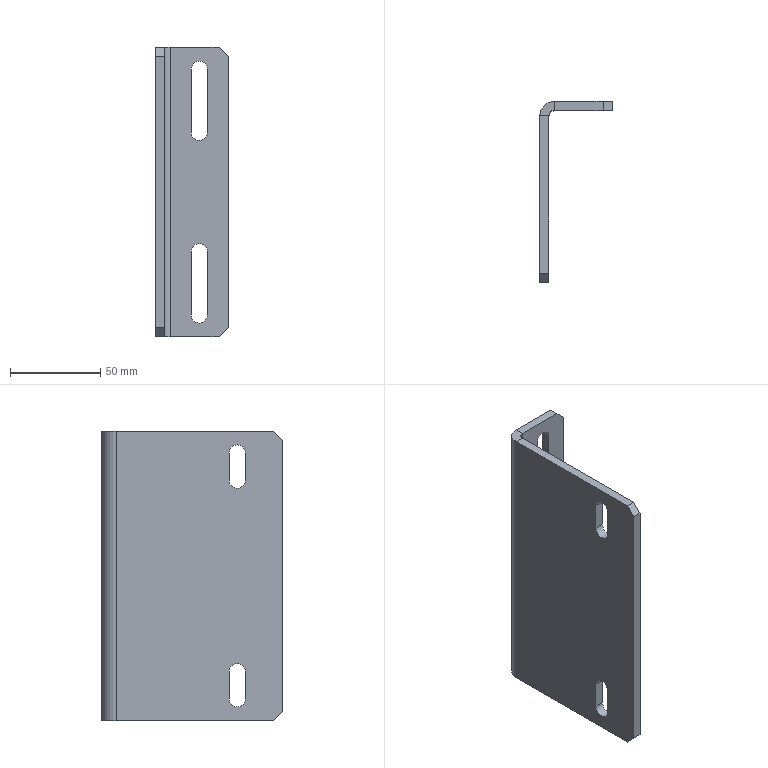Part | SolidWorks | features ICE 2, Chamfer 1, FlatPattern 1, SMBaseFlange 1, SheetMetal 1 | 1 solid | 38 faces | box 40 x 100 x 160 mm | volume 100089 mm3 | plane 24 | cylinder 14 | commonest cylinder face diameters 9 x12 6 x1 16 x1
STEP:
#1=CARTESIAN_POINT('',(28.5,100.,113.));
#2=VERTEX_POINT('',#1);
#3=CARTESIAN_POINT('',(24.,100.,108.5));
#4=VERTEX_POINT('',#3);
#5=CARTESIAN_POINT('',(24.,100.,113.));
#6=DIRECTION('',(0.,1.,0.));
#7=DIRECTION('',(0.,0.,1.));
#8=AXIS2_PLACEMENT_3D('',#5,#6,#7);
#9=CIRCLE('',#8,4.5);
#10=EDGE_CURVE('',#2,#4,#9,.T.);
#11=ORIENTED_EDGE('',*,*,#10,.T.);
#12=CARTESIAN_POINT('',(24.,95.,108.5));
#13=VERTEX_POINT('',#12);
#14=CARTESIAN_POINT('',(24.,105.,108.5));
#15=DIRECTION('',(0.,-1.,0.));
#16=VECTOR('',#15,1000.);
#17=LINE('',#14,#16);
#18=EDGE_CURVE('',#4,#13,#17,.T.);
#19=ORIENTED_EDGE('',*,*,#18,.T.);
#20=CARTESIAN_POINT('',(28.5,95.,113.));
#21=VERTEX_POINT('',#20);
#22=CARTESIAN_POINT('',(24.,95.,113.));
#23=DIRECTION('',(0.,-1.,0.));
#24=DIRECTION('',(0.,0.,1.));
#25=AXIS2_PLACEMENT_3D('',#22,#23,#24);
#26=CIRCLE('',#25,4.5);
#27=EDGE_CURVE('',#13,#21,#26,.T.);
#28=ORIENTED_EDGE('',*,*,#27,.T.);
#29=CARTESIAN_POINT('',(28.5,105.,113.));
#30=DIRECTION('',(0.,-1.,0.));
#31=VECTOR('',#30,1000.);
#32=LINE('',#29,#31);
#33=EDGE_CURVE('',#2,#21,#32,.T.);
#34=ORIENTED_EDGE('',*,*,#33,.F.);
#35=EDGE_LOOP('',(#11,#19,#28,#34));
#36=FACE_OUTER_BOUND('',#35,.T.);
#37=CARTESIAN_POINT('',(24.,105.,113.));
#38=DIRECTION('',(0.,-1.,0.));
#39=DIRECTION('',(0.,0.,-1.));
#40=AXIS2_PLACEMENT_3D('',#37,#38,#39);
#41=CYLINDRICAL_SURFACE('',#40,4.5);
#42=ADVANCED_FACE('',(#36),#41,.F.);
#43=CARTESIAN_POINT('',(28.5,100.,12.));
#44=VERTEX_POINT('',#43);
#45=CARTESIAN_POINT('',(24.,100.,7.5));
#46=VERTEX_POINT('',#45);
#47=CARTESIAN_POINT('',(24.,100.,12.));
#48=DIRECTION('',(0.,1.,0.));
#49=DIRECTION('',(0.,0.,1.));
#50=AXIS2_PLACEMENT_3D('',#47,#48,#49);
#51=CIRCLE('',#50,4.5);
#52=EDGE_CURVE('',#44,#46,#51,.T.);
#53=ORIENTED_EDGE('',*,*,#52,.T.);
#54=CARTESIAN_POINT('',(24.,95.,7.5));
#55=VERTEX_POINT('',#54);
#56=CARTESIAN_POINT('',(24.,105.,7.5));
#57=DIRECTION('',(0.,-1.,0.));
#58=VECTOR('',#57,1000.);
#59=LINE('',#56,#58);
#60=EDGE_CURVE('',#46,#55,#59,.T.);
#61=ORIENTED_EDGE('',*,*,#60,.T.);
#62=CARTESIAN_POINT('',(28.5,95.,12.));
#63=VERTEX_POINT('',#62);
#64=CARTESIAN_POINT('',(24.,95.,12.));
#65=DIRECTION('',(0.,-1.,0.));
#66=DIRECTION('',(0.,0.,-1.));
#67=AXIS2_PLACEMENT_3D('',#64,#65,#66);
#68=CIRCLE('',#67,4.5);
#69=EDGE_CURVE('',#55,#63,#68,.T.);
#70=ORIENTED_EDGE('',*,*,#69,.T.);
#71=CARTESIAN_POINT('',(28.5,105.,12.));
#72=DIRECTION('',(0.,-1.,0.));
#73=VECTOR('',#72,1000.);
#74=LINE('',#71,#73);
#75=EDGE_CURVE('',#44,#63,#74,.T.);
#76=ORIENTED_EDGE('',*,*,#75,.F.);
#77=EDGE_LOOP('',(#53,#61,#70,#76));
#78=FACE_OUTER_BOUND('',#77,.T.);
#79=CARTESIAN_POINT('',(24.,105.,12.));
#80=DIRECTION('',(0.,-1.,0.));
#81=DIRECTION('',(0.,0.,-1.));
#82=AXIS2_PLACEMENT_3D('',#79,#80,#81);
#83=CYLINDRICAL_SURFACE('',#82,4.5);
#84=ADVANCED_FACE('',(#78),#83,.F.);
#85=CARTESIAN_POINT('',(5.,25.,152.5));
#86=VERTEX_POINT('',#85);
#87=CARTESIAN_POINT('',(5.,29.5,148.));
#88=VERTEX_POINT('',#87);
#89=CARTESIAN_POINT('',(5.,25.,148.));
#90=DIRECTION('',(-1.,0.,0.));
#91=DIRECTION('',(0.,0.,1.));
#92=AXIS2_PLACEMENT_3D('',#89,#90,#91);
#93=CIRCLE('',#92,4.5);
#94=EDGE_CURVE('',#86,#88,#93,.T.);
#95=ORIENTED_EDGE('',*,*,#94,.F.);
#96=CARTESIAN_POINT('',(0.,25.,152.5));
#97=VERTEX_POINT('',#96);
#98=CARTESIAN_POINT('',(10.,25.,152.5));
#99=DIRECTION('',(-1.,0.,0.));
#100=VECTOR('',#99,1000.);
#101=LINE('',#98,#100);
#102=EDGE_CURVE('',#86,#97,#101,.T.);
#103=ORIENTED_EDGE('',*,*,#102,.T.);
#104=CARTESIAN_POINT('',(0.,29.5,148.));
#105=VERTEX_POINT('',#104);
#106=CARTESIAN_POINT('',(0.,25.,148.));
#107=DIRECTION('',(-1.,0.,0.));
#108=DIRECTION('',(0.,0.,1.));
#109=AXIS2_PLACEMENT_3D('',#106,#107,#108);
#110=CIRCLE('',#109,4.5);
#111=EDGE_CURVE('',#97,#105,#110,.T.);
#112=ORIENTED_EDGE('',*,*,#111,.T.);
#113=CARTESIAN_POINT('',(10.,29.5,148.));
#114=DIRECTION('',(-1.,0.,0.));
#115=VECTOR('',#114,1000.);
#116=LINE('',#113,#115);
#117=EDGE_CURVE('',#88,#105,#116,.T.);
#118=ORIENTED_EDGE('',*,*,#117,.F.);
#119=EDGE_LOOP('',(#95,#103,#112,#118));
#120=FACE_OUTER_BOUND('',#119,.T.);
#121=CARTESIAN_POINT('',(10.,25.,148.));
#122=DIRECTION('',(-1.,0.,0.));
#123=DIRECTION('',(0.,0.,1.));
#124=AXIS2_PLACEMENT_3D('',#121,#122,#123);
#125=CYLINDRICAL_SURFACE('',#124,4.5);
#126=ADVANCED_FACE('',(#120),#125,.F.);
#127=CARTESIAN_POINT('',(5.,25.,31.5));
#128=VERTEX_POINT('',#127);
#129=CARTESIAN_POINT('',(5.,29.5,27.));
#130=VERTEX_POINT('',#129);
#131=CARTESIAN_POINT('',(5.,25.,27.));
#132=DIRECTION('',(-1.,0.,0.));
#133=DIRECTION('',(0.,0.,1.));
#134=AXIS2_PLACEMENT_3D('',#131,#132,#133);
#135=CIRCLE('',#134,4.5);
#136=EDGE_CURVE('',#128,#130,#135,.T.);
#137=ORIENTED_EDGE('',*,*,#136,.F.);
#138=CARTESIAN_POINT('',(0.,25.,31.5));
#139=VERTEX_POINT('',#138);
#140=CARTESIAN_POINT('',(10.,25.,31.5));
#141=DIRECTION('',(-1.,0.,0.));
#142=VECTOR('',#141,1000.);
#143=LINE('',#140,#142);
#144=EDGE_CURVE('',#128,#139,#143,.T.);
#145=ORIENTED_EDGE('',*,*,#144,.T.);
#146=CARTESIAN_POINT('',(0.,29.5,27.));
#147=VERTEX_POINT('',#146);
#148=CARTESIAN_POINT('',(0.,25.,27.));
#149=DIRECTION('',(-1.,0.,0.));
#150=DIRECTION('',(0.,0.,1.));
#151=AXIS2_PLACEMENT_3D('',#148,#149,#150);
#152=CIRCLE('',#151,4.5);
#153=EDGE_CURVE('',#139,#147,#152,.T.);
#154=ORIENTED_EDGE('',*,*,#153,.T.);
#155=CARTESIAN_POINT('',(10.,29.5,27.));
#156=DIRECTION('',(-1.,0.,0.));
#157=VECTOR('',#156,1000.);
#158=LINE('',#155,#157);
#159=EDGE_CURVE('',#130,#147,#158,.T.);
#160=ORIENTED_EDGE('',*,*,#159,.F.);
#161=EDGE_LOOP('',(#137,#145,#154,#160));
#162=FACE_OUTER_BOUND('',#161,.T.);
#163=CARTESIAN_POINT('',(10.,25.,27.));
#164=DIRECTION('',(-1.,0.,0.));
#165=DIRECTION('',(0.,0.,1.));
#166=AXIS2_PLACEMENT_3D('',#163,#164,#165);
#167=CYLINDRICAL_SURFACE('',#166,4.5);
#168=ADVANCED_FACE('',(#162),#167,.F.);
#169=CARTESIAN_POINT('',(8.,100.,160.));
#170=VERTEX_POINT('',#169);
#171=CARTESIAN_POINT('',(8.,95.,160.));
#172=VERTEX_POINT('',#171);
#173=CARTESIAN_POINT('',(8.,100.,160.));
#174=DIRECTION('',(0.,-1.,0.));
#175=VECTOR('',#174,1000.);
#176=LINE('',#173,#175);
#177=EDGE_CURVE('',#170,#172,#176,.T.);
#178=ORIENTED_EDGE('',*,*,#177,.F.);
#179=CARTESIAN_POINT('',(0.,92.,160.));
#180=VERTEX_POINT('',#179);
#181=CARTESIAN_POINT('',(8.,92.,160.));
#182=DIRECTION('',(0.,0.,-1.));
#183=DIRECTION('',(1.,0.,0.));
#184=AXIS2_PLACEMENT_3D('',#181,#182,#183);
#185=CIRCLE('',#184,8.);
#186=EDGE_CURVE('',#180,#170,#185,.T.);
#187=ORIENTED_EDGE('',*,*,#186,.F.);
#188=CARTESIAN_POINT('',(5.,92.,160.));
#189=VERTEX_POINT('',#188);
#190=CARTESIAN_POINT('',(5.,92.,160.));
#191=DIRECTION('',(-1.,0.,0.));
#192=VECTOR('',#191,1000.);
#193=LINE('',#190,#192);
#194=EDGE_CURVE('',#189,#180,#193,.T.);
#195=ORIENTED_EDGE('',*,*,#194,.F.);
#196=CARTESIAN_POINT('',(8.,92.,160.));
#197=DIRECTION('',(0.,0.,-1.));
#198=DIRECTION('',(1.,0.,0.));
#199=AXIS2_PLACEMENT_3D('',#196,#197,#198);
#200=CIRCLE('',#199,3.);
#201=EDGE_CURVE('',#189,#172,#200,.T.);
#202=ORIENTED_EDGE('',*,*,#201,.T.);
#203=EDGE_LOOP('',(#178,#187,#195,#202));
#204=FACE_OUTER_BOUND('',#203,.T.);
#205=CARTESIAN_POINT('',(8.,100.,160.));
#206=DIRECTION('',(0.,0.,1.));
#207=DIRECTION('',(1.,0.,0.));
#208=AXIS2_PLACEMENT_3D('',#205,#206,#207);
#209=PLANE('',#208);
#210=ADVANCED_FACE('',(#204),#209,.T.);
#211=CARTESIAN_POINT('',(35.,95.,160.));
#212=VERTEX_POINT('',#211);
#213=CARTESIAN_POINT('',(0.,95.,160.));
#214=DIRECTION('',(1.,0.,0.));
#215=VECTOR('',#214,1000.);
#216=LINE('',#213,#215);
#217=EDGE_CURVE('',#172,#212,#216,.T.);
#218=ORIENTED_EDGE('',*,*,#217,.T.);
#219=CARTESIAN_POINT('',(35.,100.,160.));
#220=VERTEX_POINT('',#219);
#221=CARTESIAN_POINT('',(35.,92.,160.));
#222=DIRECTION('',(0.,1.,0.));
#223=VECTOR('',#222,1000.);
#224=LINE('',#221,#223);
#225=EDGE_CURVE('',#212,#220,#224,.T.);
#226=ORIENTED_EDGE('',*,*,#225,.T.);
#227=CARTESIAN_POINT('',(0.,100.,160.));
#228=DIRECTION('',(1.,0.,0.));
#229=VECTOR('',#228,1000.);
#230=LINE('',#227,#229);
#231=EDGE_CURVE('',#170,#220,#230,.T.);
#232=ORIENTED_EDGE('',*,*,#231,.F.);
#233=ORIENTED_EDGE('',*,*,#177,.T.);
#234=EDGE_LOOP('',(#218,#226,#232,#233));
#235=FACE_OUTER_BOUND('',#234,.T.);
#236=CARTESIAN_POINT('',(5.,92.,160.));
#237=DIRECTION('',(0.,0.,1.));
#238=DIRECTION('',(1.,0.,0.));
#239=AXIS2_PLACEMENT_3D('',#236,#237,#238);
#240=PLANE('',#239);
#241=ADVANCED_FACE('',(#235),#240,.T.);
#242=CARTESIAN_POINT('',(0.,92.,0.));
#243=VERTEX_POINT('',#242);
#244=CARTESIAN_POINT('',(5.,92.,0.));
#245=VERTEX_POINT('',#244);
#246=CARTESIAN_POINT('',(0.,92.,0.));
#247=DIRECTION('',(1.,0.,0.));
#248=VECTOR('',#247,1000.);
#249=LINE('',#246,#248);
#250=EDGE_CURVE('',#243,#245,#249,.T.);
#251=ORIENTED_EDGE('',*,*,#250,.F.);
#252=CARTESIAN_POINT('',(8.,100.,0.));
#253=VERTEX_POINT('',#252);
#254=CARTESIAN_POINT('',(8.,92.,0.));
#255=DIRECTION('',(0.,0.,-1.));
#256=DIRECTION('',(1.,0.,0.));
#257=AXIS2_PLACEMENT_3D('',#254,#255,#256);
#258=CIRCLE('',#257,8.);
#259=EDGE_CURVE('',#243,#253,#258,.T.);
#260=ORIENTED_EDGE('',*,*,#259,.T.);
#261=CARTESIAN_POINT('',(8.,95.,0.));
#262=VERTEX_POINT('',#261);
#263=CARTESIAN_POINT('',(8.,95.,0.));
#264=DIRECTION('',(0.,1.,0.));
#265=VECTOR('',#264,1000.);
#266=LINE('',#263,#265);
#267=EDGE_CURVE('',#262,#253,#266,.T.);
#268=ORIENTED_EDGE('',*,*,#267,.F.);
#269=CARTESIAN_POINT('',(8.,92.,0.));
#270=DIRECTION('',(0.,0.,-1.));
#271=DIRECTION('',(1.,0.,0.));
#272=AXIS2_PLACEMENT_3D('',#269,#270,#271);
#273=CIRCLE('',#272,3.);
#274=EDGE_CURVE('',#245,#262,#273,.T.);
#275=ORIENTED_EDGE('',*,*,#274,.F.);
#276=EDGE_LOOP('',(#251,#260,#268,#275));
#277=FACE_OUTER_BOUND('',#276,.T.);
#278=CARTESIAN_POINT('',(0.,92.,0.));
#279=DIRECTION('',(0.,0.,-1.));
#280=DIRECTION('',(-1.,0.,0.));
#281=AXIS2_PLACEMENT_3D('',#278,#279,#280);
#282=PLANE('',#281);
#283=ADVANCED_FACE('',(#277),#282,.T.);
#284=CARTESIAN_POINT('',(5.,5.,0.));
#285=VERTEX_POINT('',#284);
#286=CARTESIAN_POINT('',(5.,0.,0.));
#287=DIRECTION('',(0.,1.,0.));
#288=VECTOR('',#287,1000.);
#289=LINE('',#286,#288);
#290=EDGE_CURVE('',#285,#245,#289,.T.);
#291=ORIENTED_EDGE('',*,*,#290,.F.);
#292=CARTESIAN_POINT('',(0.,5.,0.));
#293=VERTEX_POINT('',#292);
#294=CARTESIAN_POINT('',(8.,5.,0.));
#295=DIRECTION('',(-1.,0.,0.));
#296=VECTOR('',#295,1000.);
#297=LINE('',#294,#296);
#298=EDGE_CURVE('',#285,#293,#297,.T.);
#299=ORIENTED_EDGE('',*,*,#298,.T.);
#300=CARTESIAN_POINT('',(0.,0.,0.));
#301=DIRECTION('',(0.,1.,0.));
#302=VECTOR('',#301,1000.);
#303=LINE('',#300,#302);
#304=EDGE_CURVE('',#293,#243,#303,.T.);
#305=ORIENTED_EDGE('',*,*,#304,.T.);
#306=ORIENTED_EDGE('',*,*,#250,.T.);
#307=EDGE_LOOP('',(#291,#299,#305,#306));
#308=FACE_OUTER_BOUND('',#307,.T.);
#309=CARTESIAN_POINT('',(8.,95.,0.));
#310=DIRECTION('',(0.,0.,-1.));
#311=DIRECTION('',(-1.,0.,0.));
#312=AXIS2_PLACEMENT_3D('',#309,#310,#311);
#313=PLANE('',#312);
#314=ADVANCED_FACE('',(#308),#313,.T.);
#315=CARTESIAN_POINT('',(19.5,95.,148.));
#316=VERTEX_POINT('',#315);
#317=CARTESIAN_POINT('',(19.5,95.,113.));
#318=VERTEX_POINT('',#317);
#319=CARTESIAN_POINT('',(19.5,95.,148.));
#320=DIRECTION('',(0.,0.,-1.));
#321=VECTOR('',#320,1000.);
#322=LINE('',#319,#321);
#323=EDGE_CURVE('',#316,#318,#322,.T.);
#324=ORIENTED_EDGE('',*,*,#323,.F.);
#325=CARTESIAN_POINT('',(28.5,95.,148.));
#326=VERTEX_POINT('',#325);
#327=CARTESIAN_POINT('',(24.,95.,148.));
#328=DIRECTION('',(0.,-1.,0.));
#329=DIRECTION('',(0.,0.,1.));
#330=AXIS2_PLACEMENT_3D('',#327,#328,#329);
#331=CIRCLE('',#330,4.5);
#332=EDGE_CURVE('',#326,#316,#331,.T.);
#333=ORIENTED_EDGE('',*,*,#332,.F.);
#334=CARTESIAN_POINT('',(28.5,95.,148.));
#335=DIRECTION('',(0.,0.,1.));
#336=VECTOR('',#335,1000.);
#337=LINE('',#334,#336);
#338=EDGE_CURVE('',#21,#326,#337,.T.);
#339=ORIENTED_EDGE('',*,*,#338,.F.);
#340=ORIENTED_EDGE('',*,*,#27,.F.);
#341=CARTESIAN_POINT('',(24.,95.,113.));
#342=DIRECTION('',(0.,-1.,0.));
#343=DIRECTION('',(0.,0.,1.));
#344=AXIS2_PLACEMENT_3D('',#341,#342,#343);
#345=CIRCLE('',#344,4.5);
#346=EDGE_CURVE('',#318,#13,#345,.T.);
#347=ORIENTED_EDGE('',*,*,#346,.F.);
#348=EDGE_LOOP('',(#324,#333,#339,#340,#347));
#349=FACE_BOUND('',#348,.T.);
#350=CARTESIAN_POINT('',(28.5,95.,47.));
#351=VERTEX_POINT('',#350);
#352=CARTESIAN_POINT('',(28.5,95.,12.));
#353=DIRECTION('',(0.,0.,1.));
#354=VECTOR('',#353,1000.);
#355=LINE('',#352,#354);
#356=EDGE_CURVE('',#63,#351,#355,.T.);
#357=ORIENTED_EDGE('',*,*,#356,.F.);
#358=ORIENTED_EDGE('',*,*,#69,.F.);
#359=CARTESIAN_POINT('',(19.5,95.,12.));
#360=VERTEX_POINT('',#359);
#361=CARTESIAN_POINT('',(24.,95.,12.));
#362=DIRECTION('',(0.,-1.,0.));
#363=DIRECTION('',(0.,0.,-1.));
#364=AXIS2_PLACEMENT_3D('',#361,#362,#363);
#365=CIRCLE('',#364,4.5);
#366=EDGE_CURVE('',#360,#55,#365,.T.);
#367=ORIENTED_EDGE('',*,*,#366,.F.);
#368=CARTESIAN_POINT('',(19.5,95.,47.));
#369=VERTEX_POINT('',#368);
#370=CARTESIAN_POINT('',(19.5,95.,12.));
#371=DIRECTION('',(0.,0.,-1.));
#372=VECTOR('',#371,1000.);
#373=LINE('',#370,#372);
#374=EDGE_CURVE('',#369,#360,#373,.T.);
#375=ORIENTED_EDGE('',*,*,#374,.F.);
#376=CARTESIAN_POINT('',(24.,95.,47.));
#377=DIRECTION('',(0.,-1.,0.));
#378=DIRECTION('',(0.,0.,-1.));
#379=AXIS2_PLACEMENT_3D('',#376,#377,#378);
#380=CIRCLE('',#379,4.5);
#381=EDGE_CURVE('',#351,#369,#380,.T.);
#382=ORIENTED_EDGE('',*,*,#381,.F.);
#383=EDGE_LOOP('',(#357,#358,#367,#375,#382));
#384=FACE_BOUND('',#383,.T.);
#385=CARTESIAN_POINT('',(35.,95.,0.));
#386=VERTEX_POINT('',#385);
#387=CARTESIAN_POINT('',(0.,95.,0.));
#388=DIRECTION('',(1.,0.,0.));
#389=VECTOR('',#388,1000.);
#390=LINE('',#387,#389);
#391=EDGE_CURVE('',#262,#386,#390,.T.);
#392=ORIENTED_EDGE('',*,*,#391,.T.);
#393=CARTESIAN_POINT('',(40.,95.,5.));
#394=VERTEX_POINT('',#393);
#395=CARTESIAN_POINT('',(35.,95.,0.));
#396=DIRECTION('',(0.7071,0.,0.7071));
#397=VECTOR('',#396,1000.);
#398=LINE('',#395,#397);
#399=EDGE_CURVE('',#386,#394,#398,.T.);
#400=ORIENTED_EDGE('',*,*,#399,.T.);
#401=CARTESIAN_POINT('',(40.,95.,155.));
#402=VERTEX_POINT('',#401);
#403=CARTESIAN_POINT('',(40.,95.,160.));
#404=DIRECTION('',(0.,0.,-1.));
#405=VECTOR('',#404,1000.);
#406=LINE('',#403,#405);
#407=EDGE_CURVE('',#402,#394,#406,.T.);
#408=ORIENTED_EDGE('',*,*,#407,.F.);
#409=CARTESIAN_POINT('',(40.,95.,155.));
#410=DIRECTION('',(-0.7071,0.,0.7071));
#411=VECTOR('',#410,1000.);
#412=LINE('',#409,#411);
#413=EDGE_CURVE('',#402,#212,#412,.T.);
#414=ORIENTED_EDGE('',*,*,#413,.T.);
#415=ORIENTED_EDGE('',*,*,#217,.F.);
#416=CARTESIAN_POINT('',(8.,95.,160.));
#417=DIRECTION('',(0.,0.,-1.));
#418=VECTOR('',#417,1000.);
#419=LINE('',#416,#418);
#420=EDGE_CURVE('',#172,#262,#419,.T.);
#421=ORIENTED_EDGE('',*,*,#420,.T.);
#422=EDGE_LOOP('',(#392,#400,#408,#414,#415,#421));
#423=FACE_OUTER_BOUND('',#422,.T.);
#424=CARTESIAN_POINT('',(0.,95.,160.));
#425=DIRECTION('',(0.,1.,0.));
#426=DIRECTION('',(0.,0.,1.));
#427=AXIS2_PLACEMENT_3D('',#424,#425,#426);
#428=PLANE('',#427);
#429=ADVANCED_FACE('',(#349,#384,#423),#428,.F.);
#430=ORIENTED_EDGE('',*,*,#407,.T.);
#431=CARTESIAN_POINT('',(40.,100.,5.));
#432=VERTEX_POINT('',#431);
#433=CARTESIAN_POINT('',(40.,100.,5.));
#434=DIRECTION('',(0.,1.,0.));
#435=VECTOR('',#434,1000.);
#436=LINE('',#433,#435);
#437=EDGE_CURVE('',#394,#432,#436,.T.);
#438=ORIENTED_EDGE('',*,*,#437,.T.);
#439=CARTESIAN_POINT('',(40.,100.,155.));
#440=VERTEX_POINT('',#439);
#441=CARTESIAN_POINT('',(40.,100.,160.));
#442=DIRECTION('',(0.,0.,-1.));
#443=VECTOR('',#442,1000.);
#444=LINE('',#441,#443);
#445=EDGE_CURVE('',#440,#432,#444,.T.);
#446=ORIENTED_EDGE('',*,*,#445,.F.);
#447=CARTESIAN_POINT('',(40.,100.,155.));
#448=DIRECTION('',(0.,-1.,0.));
#449=VECTOR('',#448,1000.);
#450=LINE('',#447,#449);
#451=EDGE_CURVE('',#440,#402,#450,.T.);
#452=ORIENTED_EDGE('',*,*,#451,.T.);
#453=EDGE_LOOP('',(#430,#438,#446,#452));
#454=FACE_OUTER_BOUND('',#453,.T.);
#455=CARTESIAN_POINT('',(40.,100.,160.));
#456=DIRECTION('',(1.,0.,0.));
#457=DIRECTION('',(0.,0.,-1.));
#458=AXIS2_PLACEMENT_3D('',#455,#456,#457);
#459=PLANE('',#458);
#460=ADVANCED_FACE('',(#454),#459,.T.);
#461=CARTESIAN_POINT('',(19.5,100.,148.));
#462=VERTEX_POINT('',#461);
#463=CARTESIAN_POINT('',(28.5,100.,148.));
#464=VERTEX_POINT('',#463);
#465=CARTESIAN_POINT('',(24.,100.,148.));
#466=DIRECTION('',(0.,1.,0.));
#467=DIRECTION('',(0.,0.,1.));
#468=AXIS2_PLACEMENT_3D('',#465,#466,#467);
#469=CIRCLE('',#468,4.5);
#470=EDGE_CURVE('',#462,#464,#469,.T.);
#471=ORIENTED_EDGE('',*,*,#470,.F.);
#472=CARTESIAN_POINT('',(19.5,100.,113.));
#473=VERTEX_POINT('',#472);
#474=CARTESIAN_POINT('',(19.5,100.,160.));
#475=DIRECTION('',(0.,0.,1.));
#476=VECTOR('',#475,1000.);
#477=LINE('',#474,#476);
#478=EDGE_CURVE('',#473,#462,#477,.T.);
#479=ORIENTED_EDGE('',*,*,#478,.F.);
#480=CARTESIAN_POINT('',(24.,100.,113.));
#481=DIRECTION('',(0.,1.,0.));
#482=DIRECTION('',(0.,0.,1.));
#483=AXIS2_PLACEMENT_3D('',#480,#481,#482);
#484=CIRCLE('',#483,4.5);
#485=EDGE_CURVE('',#4,#473,#484,.T.);
#486=ORIENTED_EDGE('',*,*,#485,.F.);
#487=ORIENTED_EDGE('',*,*,#10,.F.);
#488=CARTESIAN_POINT('',(28.5,100.,160.));
#489=DIRECTION('',(0.,0.,-1.));
#490=VECTOR('',#489,1000.);
#491=LINE('',#488,#490);
#492=EDGE_CURVE('',#464,#2,#491,.T.);
#493=ORIENTED_EDGE('',*,*,#492,.F.);
#494=EDGE_LOOP('',(#471,#479,#486,#487,#493));
#495=FACE_BOUND('',#494,.T.);
#496=ORIENTED_EDGE('',*,*,#52,.F.);
#497=CARTESIAN_POINT('',(28.5,100.,47.));
#498=VERTEX_POINT('',#497);
#499=CARTESIAN_POINT('',(28.5,100.,160.));
#500=DIRECTION('',(0.,0.,-1.));
#501=VECTOR('',#500,1000.);
#502=LINE('',#499,#501);
#503=EDGE_CURVE('',#498,#44,#502,.T.);
#504=ORIENTED_EDGE('',*,*,#503,.F.);
#505=CARTESIAN_POINT('',(19.5,100.,47.));
#506=VERTEX_POINT('',#505);
#507=CARTESIAN_POINT('',(24.,100.,47.));
#508=DIRECTION('',(0.,1.,0.));
#509=DIRECTION('',(0.,0.,1.));
#510=AXIS2_PLACEMENT_3D('',#507,#508,#509);
#511=CIRCLE('',#510,4.5);
#512=EDGE_CURVE('',#506,#498,#511,.T.);
#513=ORIENTED_EDGE('',*,*,#512,.F.);
#514=CARTESIAN_POINT('',(19.5,100.,12.));
#515=VERTEX_POINT('',#514);
#516=CARTESIAN_POINT('',(19.5,100.,160.));
#517=DIRECTION('',(0.,0.,1.));
#518=VECTOR('',#517,1000.);
#519=LINE('',#516,#518);
#520=EDGE_CURVE('',#515,#506,#519,.T.);
#521=ORIENTED_EDGE('',*,*,#520,.F.);
#522=CARTESIAN_POINT('',(24.,100.,12.));
#523=DIRECTION('',(0.,1.,0.));
#524=DIRECTION('',(0.,0.,1.));
#525=AXIS2_PLACEMENT_3D('',#522,#523,#524);
#526=CIRCLE('',#525,4.5);
#527=EDGE_CURVE('',#46,#515,#526,.T.);
#528=ORIENTED_EDGE('',*,*,#527,.F.);
#529=EDGE_LOOP('',(#496,#504,#513,#521,#528));
#530=FACE_BOUND('',#529,.T.);
#531=ORIENTED_EDGE('',*,*,#445,.T.);
#532=CARTESIAN_POINT('',(35.,100.,0.));
#533=VERTEX_POINT('',#532);
#534=CARTESIAN_POINT('',(97.5,100.,62.5));
#535=DIRECTION('',(-0.7071,0.,-0.7071));
#536=VECTOR('',#535,1000.);
#537=LINE('',#534,#536);
#538=EDGE_CURVE('',#432,#533,#537,.T.);
#539=ORIENTED_EDGE('',*,*,#538,.T.);
#540=CARTESIAN_POINT('',(0.,100.,0.));
#541=DIRECTION('',(1.,0.,0.));
#542=VECTOR('',#541,1000.);
#543=LINE('',#540,#542);
#544=EDGE_CURVE('',#253,#533,#543,.T.);
#545=ORIENTED_EDGE('',*,*,#544,.F.);
#546=CARTESIAN_POINT('',(8.,100.,160.));
#547=DIRECTION('',(0.,0.,-1.));
#548=VECTOR('',#547,1000.);
#549=LINE('',#546,#548);
#550=EDGE_CURVE('',#170,#253,#549,.T.);
#551=ORIENTED_EDGE('',*,*,#550,.F.);
#552=ORIENTED_EDGE('',*,*,#231,.T.);
#553=CARTESIAN_POINT('',(17.5,100.,177.5));
#554=DIRECTION('',(0.7071,0.,-0.7071));
#555=VECTOR('',#554,1000.);
#556=LINE('',#553,#555);
#557=EDGE_CURVE('',#220,#440,#556,.T.);
#558=ORIENTED_EDGE('',*,*,#557,.T.);
#559=EDGE_LOOP('',(#531,#539,#545,#551,#552,#558));
#560=FACE_OUTER_BOUND('',#559,.T.);
#561=CARTESIAN_POINT('',(0.,100.,160.));
#562=DIRECTION('',(0.,1.,0.));
#563=DIRECTION('',(0.,0.,1.));
#564=AXIS2_PLACEMENT_3D('',#561,#562,#563);
#565=PLANE('',#564);
#566=ADVANCED_FACE('',(#495,#530,#560),#565,.T.);
#567=ORIENTED_EDGE('',*,*,#259,.F.);
#568=CARTESIAN_POINT('',(0.,92.,160.));
#569=DIRECTION('',(0.,0.,-1.));
#570=VECTOR('',#569,1000.);
#571=LINE('',#568,#570);
#572=EDGE_CURVE('',#180,#243,#571,.T.);
#573=ORIENTED_EDGE('',*,*,#572,.F.);
#574=ORIENTED_EDGE('',*,*,#186,.T.);
#575=ORIENTED_EDGE('',*,*,#550,.T.);
#576=EDGE_LOOP('',(#567,#573,#574,#575));
#577=FACE_OUTER_BOUND('',#576,.T.);
#578=CARTESIAN_POINT('',(8.,92.,160.));
#579=DIRECTION('',(0.,0.,-1.));
#580=DIRECTION('',(-1.,0.,0.));
#581=AXIS2_PLACEMENT_3D('',#578,#579,#580);
#582=CYLINDRICAL_SURFACE('',#581,8.);
#583=ADVANCED_FACE('',(#577),#582,.T.);
#584=CARTESIAN_POINT('',(0.,20.5,148.));
#585=VERTEX_POINT('',#584);
#586=CARTESIAN_POINT('',(0.,25.,148.));
#587=DIRECTION('',(-1.,0.,0.));
#588=DIRECTION('',(0.,0.,1.));
#589=AXIS2_PLACEMENT_3D('',#586,#587,#588);
#590=CIRCLE('',#589,4.5);
#591=EDGE_CURVE('',#585,#97,#590,.T.);
#592=ORIENTED_EDGE('',*,*,#591,.F.);
#593=CARTESIAN_POINT('',(0.,20.5,133.));
#594=VERTEX_POINT('',#593);
#595=CARTESIAN_POINT('',(0.,20.5,148.));
#596=DIRECTION('',(0.,0.,1.));
#597=VECTOR('',#596,1000.);
#598=LINE('',#595,#597);
#599=EDGE_CURVE('',#594,#585,#598,.T.);
#600=ORIENTED_EDGE('',*,*,#599,.F.);
#601=CARTESIAN_POINT('',(0.,29.5,133.));
#602=VERTEX_POINT('',#601);
#603=CARTESIAN_POINT('',(0.,25.,133.));
#604=DIRECTION('',(-1.,0.,0.));
#605=DIRECTION('',(0.,0.,1.));
#606=AXIS2_PLACEMENT_3D('',#603,#604,#605);
#607=CIRCLE('',#606,4.5);
#608=EDGE_CURVE('',#602,#594,#607,.T.);
#609=ORIENTED_EDGE('',*,*,#608,.F.);
#610=CARTESIAN_POINT('',(0.,29.5,148.));
#611=DIRECTION('',(0.,0.,-1.));
#612=VECTOR('',#611,1000.);
#613=LINE('',#610,#612);
#614=EDGE_CURVE('',#105,#602,#613,.T.);
#615=ORIENTED_EDGE('',*,*,#614,.F.);
#616=ORIENTED_EDGE('',*,*,#111,.F.);
#617=EDGE_LOOP('',(#592,#600,#609,#615,#616));
#618=FACE_BOUND('',#617,.T.);
#619=CARTESIAN_POINT('',(0.,29.5,12.));
#620=VERTEX_POINT('',#619);
#621=CARTESIAN_POINT('',(0.,20.5,12.));
#622=VERTEX_POINT('',#621);
#623=CARTESIAN_POINT('',(0.,25.,12.));
#624=DIRECTION('',(-1.,0.,0.));
#625=DIRECTION('',(0.,0.,1.));
#626=AXIS2_PLACEMENT_3D('',#623,#624,#625);
#627=CIRCLE('',#626,4.5);
#628=EDGE_CURVE('',#620,#622,#627,.T.);
#629=ORIENTED_EDGE('',*,*,#628,.F.);
#630=CARTESIAN_POINT('',(0.,29.5,12.));
#631=DIRECTION('',(0.,0.,-1.));
#632=VECTOR('',#631,1000.);
#633=LINE('',#630,#632);
#634=EDGE_CURVE('',#147,#620,#633,.T.);
#635=ORIENTED_EDGE('',*,*,#634,.F.);
#636=ORIENTED_EDGE('',*,*,#153,.F.);
#637=CARTESIAN_POINT('',(0.,20.5,27.));
#638=VERTEX_POINT('',#637);
#639=CARTESIAN_POINT('',(0.,25.,27.));
#640=DIRECTION('',(-1.,0.,0.));
#641=DIRECTION('',(0.,0.,1.));
#642=AXIS2_PLACEMENT_3D('',#639,#640,#641);
#643=CIRCLE('',#642,4.5);
#644=EDGE_CURVE('',#638,#139,#643,.T.);
#645=ORIENTED_EDGE('',*,*,#644,.F.);
#646=CARTESIAN_POINT('',(0.,20.5,12.));
#647=DIRECTION('',(0.,0.,1.));
#648=VECTOR('',#647,1000.);
#649=LINE('',#646,#648);
#650=EDGE_CURVE('',#622,#638,#649,.T.);
#651=ORIENTED_EDGE('',*,*,#650,.F.);
#652=EDGE_LOOP('',(#629,#635,#636,#645,#651));
#653=FACE_BOUND('',#652,.T.);
#654=ORIENTED_EDGE('',*,*,#304,.F.);
#655=CARTESIAN_POINT('',(0.,0.,5.));
#656=VERTEX_POINT('',#655);
#657=CARTESIAN_POINT('',(0.,-77.5,82.5));
#658=DIRECTION('',(0.,-0.7071,0.7071));
#659=VECTOR('',#658,1000.);
#660=LINE('',#657,#659);
#661=EDGE_CURVE('',#293,#656,#660,.T.);
#662=ORIENTED_EDGE('',*,*,#661,.T.);
#663=CARTESIAN_POINT('',(0.,0.,155.));
#664=VERTEX_POINT('',#663);
#665=CARTESIAN_POINT('',(0.,0.,160.));
#666=DIRECTION('',(0.,0.,-1.));
#667=VECTOR('',#666,1000.);
#668=LINE('',#665,#667);
#669=EDGE_CURVE('',#664,#656,#668,.T.);
#670=ORIENTED_EDGE('',*,*,#669,.F.);
#671=CARTESIAN_POINT('',(0.,5.,160.));
#672=VERTEX_POINT('',#671);
#673=CARTESIAN_POINT('',(0.,2.5,157.5));
#674=DIRECTION('',(0.,0.7071,0.7071));
#675=VECTOR('',#674,1000.);
#676=LINE('',#673,#675);
#677=EDGE_CURVE('',#664,#672,#676,.T.);
#678=ORIENTED_EDGE('',*,*,#677,.T.);
#679=CARTESIAN_POINT('',(0.,0.,160.));
#680=DIRECTION('',(0.,1.,0.));
#681=VECTOR('',#680,1000.);
#682=LINE('',#679,#681);
#683=EDGE_CURVE('',#672,#180,#682,.T.);
#684=ORIENTED_EDGE('',*,*,#683,.T.);
#685=ORIENTED_EDGE('',*,*,#572,.T.);
#686=EDGE_LOOP('',(#654,#662,#670,#678,#684,#685));
#687=FACE_OUTER_BOUND('',#686,.T.);
#688=CARTESIAN_POINT('',(0.,0.,160.));
#689=DIRECTION('',(-1.,0.,0.));
#690=DIRECTION('',(0.,0.,1.));
#691=AXIS2_PLACEMENT_3D('',#688,#689,#690);
#692=PLANE('',#691);
#693=ADVANCED_FACE('',(#618,#653,#687),#692,.T.);
#694=ORIENTED_EDGE('',*,*,#669,.T.);
#695=CARTESIAN_POINT('',(5.,0.,5.));
#696=VERTEX_POINT('',#695);
#697=CARTESIAN_POINT('',(5.,0.,5.));
#698=DIRECTION('',(1.,0.,0.));
#699=VECTOR('',#698,1000.);
#700=LINE('',#697,#699);
#701=EDGE_CURVE('',#656,#696,#700,.T.);
#702=ORIENTED_EDGE('',*,*,#701,.T.);
#703=CARTESIAN_POINT('',(5.,0.,155.));
#704=VERTEX_POINT('',#703);
#705=CARTESIAN_POINT('',(5.,0.,160.));
#706=DIRECTION('',(0.,0.,-1.));
#707=VECTOR('',#706,1000.);
#708=LINE('',#705,#707);
#709=EDGE_CURVE('',#704,#696,#708,.T.);
#710=ORIENTED_EDGE('',*,*,#709,.F.);
#711=CARTESIAN_POINT('',(5.,0.,155.));
#712=DIRECTION('',(-1.,0.,0.));
#713=VECTOR('',#712,1000.);
#714=LINE('',#711,#713);
#715=EDGE_CURVE('',#704,#664,#714,.T.);
#716=ORIENTED_EDGE('',*,*,#715,.T.);
#717=EDGE_LOOP('',(#694,#702,#710,#716));
#718=FACE_OUTER_BOUND('',#717,.T.);
#719=CARTESIAN_POINT('',(5.,0.,160.));
#720=DIRECTION('',(0.,-1.,0.));
#721=DIRECTION('',(0.,0.,-1.));
#722=AXIS2_PLACEMENT_3D('',#719,#720,#721);
#723=PLANE('',#722);
#724=ADVANCED_FACE('',(#718),#723,.T.);
#725=CARTESIAN_POINT('',(5.,20.5,133.));
#726=VERTEX_POINT('',#725);
#727=CARTESIAN_POINT('',(5.,20.5,148.));
#728=VERTEX_POINT('',#727);
#729=CARTESIAN_POINT('',(5.,20.5,160.));
#730=DIRECTION('',(0.,0.,1.));
#731=VECTOR('',#730,1000.);
#732=LINE('',#729,#731);
#733=EDGE_CURVE('',#726,#728,#732,.T.);
#734=ORIENTED_EDGE('',*,*,#733,.T.);
#735=CARTESIAN_POINT('',(5.,25.,148.));
#736=DIRECTION('',(-1.,0.,0.));
#737=DIRECTION('',(0.,0.,1.));
#738=AXIS2_PLACEMENT_3D('',#735,#736,#737);
#739=CIRCLE('',#738,4.5);
#740=EDGE_CURVE('',#728,#86,#739,.T.);
#741=ORIENTED_EDGE('',*,*,#740,.T.);
#742=ORIENTED_EDGE('',*,*,#94,.T.);
#743=CARTESIAN_POINT('',(5.,29.5,133.));
#744=VERTEX_POINT('',#743);
#745=CARTESIAN_POINT('',(5.,29.5,160.));
#746=DIRECTION('',(0.,0.,-1.));
#747=VECTOR('',#746,1000.);
#748=LINE('',#745,#747);
#749=EDGE_CURVE('',#88,#744,#748,.T.);
#750=ORIENTED_EDGE('',*,*,#749,.T.);
#751=CARTESIAN_POINT('',(5.,25.,133.));
#752=DIRECTION('',(-1.,0.,0.));
#753=DIRECTION('',(0.,0.,1.));
#754=AXIS2_PLACEMENT_3D('',#751,#752,#753);
#755=CIRCLE('',#754,4.5);
#756=EDGE_CURVE('',#744,#726,#755,.T.);
#757=ORIENTED_EDGE('',*,*,#756,.T.);
#758=EDGE_LOOP('',(#734,#741,#742,#750,#757));
#759=FACE_BOUND('',#758,.T.);
#760=CARTESIAN_POINT('',(5.,29.5,12.));
#761=VERTEX_POINT('',#760);
#762=CARTESIAN_POINT('',(5.,29.5,160.));
#763=DIRECTION('',(0.,0.,-1.));
#764=VECTOR('',#763,1000.);
#765=LINE('',#762,#764);
#766=EDGE_CURVE('',#130,#761,#765,.T.);
#767=ORIENTED_EDGE('',*,*,#766,.T.);
#768=CARTESIAN_POINT('',(5.,20.5,12.));
#769=VERTEX_POINT('',#768);
#770=CARTESIAN_POINT('',(5.,25.,12.));
#771=DIRECTION('',(-1.,0.,0.));
#772=DIRECTION('',(0.,0.,1.));
#773=AXIS2_PLACEMENT_3D('',#770,#771,#772);
#774=CIRCLE('',#773,4.5);
#775=EDGE_CURVE('',#761,#769,#774,.T.);
#776=ORIENTED_EDGE('',*,*,#775,.T.);
#777=CARTESIAN_POINT('',(5.,20.5,27.));
#778=VERTEX_POINT('',#777);
#779=CARTESIAN_POINT('',(5.,20.5,160.));
#780=DIRECTION('',(0.,0.,1.));
#781=VECTOR('',#780,1000.);
#782=LINE('',#779,#781);
#783=EDGE_CURVE('',#769,#778,#782,.T.);
#784=ORIENTED_EDGE('',*,*,#783,.T.);
#785=CARTESIAN_POINT('',(5.,25.,27.));
#786=DIRECTION('',(-1.,0.,0.));
#787=DIRECTION('',(0.,0.,1.));
#788=AXIS2_PLACEMENT_3D('',#785,#786,#787);
#789=CIRCLE('',#788,4.5);
#790=EDGE_CURVE('',#778,#128,#789,.T.);
#791=ORIENTED_EDGE('',*,*,#790,.T.);
#792=ORIENTED_EDGE('',*,*,#136,.T.);
#793=EDGE_LOOP('',(#767,#776,#784,#791,#792));
#794=FACE_BOUND('',#793,.T.);
#795=ORIENTED_EDGE('',*,*,#709,.T.);
#796=CARTESIAN_POINT('',(5.,5.,0.));
#797=DIRECTION('',(0.,0.7071,-0.7071));
#798=VECTOR('',#797,1000.);
#799=LINE('',#796,#798);
#800=EDGE_CURVE('',#696,#285,#799,.T.);
#801=ORIENTED_EDGE('',*,*,#800,.T.);
#802=ORIENTED_EDGE('',*,*,#290,.T.);
#803=CARTESIAN_POINT('',(5.,92.,160.));
#804=DIRECTION('',(0.,0.,-1.));
#805=VECTOR('',#804,1000.);
#806=LINE('',#803,#805);
#807=EDGE_CURVE('',#189,#245,#806,.T.);
#808=ORIENTED_EDGE('',*,*,#807,.F.);
#809=CARTESIAN_POINT('',(5.,5.,160.));
#810=VERTEX_POINT('',#809);
#811=CARTESIAN_POINT('',(5.,0.,160.));
#812=DIRECTION('',(0.,1.,0.));
#813=VECTOR('',#812,1000.);
#814=LINE('',#811,#813);
#815=EDGE_CURVE('',#810,#189,#814,.T.);
#816=ORIENTED_EDGE('',*,*,#815,.F.);
#817=CARTESIAN_POINT('',(5.,0.,155.));
#818=DIRECTION('',(0.,-0.7071,-0.7071));
#819=VECTOR('',#818,1000.);
#820=LINE('',#817,#819);
#821=EDGE_CURVE('',#810,#704,#820,.T.);
#822=ORIENTED_EDGE('',*,*,#821,.T.);
#823=EDGE_LOOP('',(#795,#801,#802,#808,#816,#822));
#824=FACE_OUTER_BOUND('',#823,.T.);
#825=CARTESIAN_POINT('',(5.,0.,160.));
#826=DIRECTION('',(-1.,0.,0.));
#827=DIRECTION('',(0.,0.,1.));
#828=AXIS2_PLACEMENT_3D('',#825,#826,#827);
#829=PLANE('',#828);
#830=ADVANCED_FACE('',(#759,#794,#824),#829,.F.);
#831=ORIENTED_EDGE('',*,*,#274,.T.);
#832=ORIENTED_EDGE('',*,*,#420,.F.);
#833=ORIENTED_EDGE('',*,*,#201,.F.);
#834=ORIENTED_EDGE('',*,*,#807,.T.);
#835=EDGE_LOOP('',(#831,#832,#833,#834));
#836=FACE_OUTER_BOUND('',#835,.T.);
#837=CARTESIAN_POINT('',(8.,92.,160.));
#838=DIRECTION('',(0.,0.,-1.));
#839=DIRECTION('',(-1.,0.,0.));
#840=AXIS2_PLACEMENT_3D('',#837,#838,#839);
#841=CYLINDRICAL_SURFACE('',#840,3.);
#842=ADVANCED_FACE('',(#836),#841,.F.);
#843=ORIENTED_EDGE('',*,*,#683,.F.);
#844=CARTESIAN_POINT('',(8.,5.,160.));
#845=DIRECTION('',(1.,0.,0.));
#846=VECTOR('',#845,1000.);
#847=LINE('',#844,#846);
#848=EDGE_CURVE('',#672,#810,#847,.T.);
#849=ORIENTED_EDGE('',*,*,#848,.T.);
#850=ORIENTED_EDGE('',*,*,#815,.T.);
#851=ORIENTED_EDGE('',*,*,#194,.T.);
#852=EDGE_LOOP('',(#843,#849,#850,#851));
#853=FACE_OUTER_BOUND('',#852,.T.);
#854=CARTESIAN_POINT('',(8.,92.,160.));
#855=DIRECTION('',(0.,0.,1.));
#856=DIRECTION('',(1.,0.,0.));
#857=AXIS2_PLACEMENT_3D('',#854,#855,#856);
#858=PLANE('',#857);
#859=ADVANCED_FACE('',(#853),#858,.T.);
#860=ORIENTED_EDGE('',*,*,#544,.T.);
#861=CARTESIAN_POINT('',(35.,95.,0.));
#862=DIRECTION('',(0.,-1.,0.));
#863=VECTOR('',#862,1000.);
#864=LINE('',#861,#863);
#865=EDGE_CURVE('',#533,#386,#864,.T.);
#866=ORIENTED_EDGE('',*,*,#865,.T.);
#867=ORIENTED_EDGE('',*,*,#391,.F.);
#868=ORIENTED_EDGE('',*,*,#267,.T.);
#869=EDGE_LOOP('',(#860,#866,#867,#868));
#870=FACE_OUTER_BOUND('',#869,.T.);
#871=CARTESIAN_POINT('',(8.,92.,0.));
#872=DIRECTION('',(0.,0.,1.));
#873=DIRECTION('',(1.,0.,0.));
#874=AXIS2_PLACEMENT_3D('',#871,#872,#873);
#875=PLANE('',#874);
#876=ADVANCED_FACE('',(#870),#875,.F.);
#877=ORIENTED_EDGE('',*,*,#538,.F.);
#878=ORIENTED_EDGE('',*,*,#437,.F.);
#879=ORIENTED_EDGE('',*,*,#399,.F.);
#880=ORIENTED_EDGE('',*,*,#865,.F.);
#881=EDGE_LOOP('',(#877,#878,#879,#880));
#882=FACE_OUTER_BOUND('',#881,.T.);
#883=CARTESIAN_POINT('',(35.,92.,0.));
#884=DIRECTION('',(0.7071,0.,-0.7071));
#885=DIRECTION('',(0.,1.,0.));
#886=AXIS2_PLACEMENT_3D('',#883,#884,#885);
#887=PLANE('',#886);
#888=ADVANCED_FACE('',(#882),#887,.T.);
#889=ORIENTED_EDGE('',*,*,#800,.F.);
#890=ORIENTED_EDGE('',*,*,#701,.F.);
#891=ORIENTED_EDGE('',*,*,#661,.F.);
#892=ORIENTED_EDGE('',*,*,#298,.F.);
#893=EDGE_LOOP('',(#889,#890,#891,#892));
#894=FACE_OUTER_BOUND('',#893,.T.);
#895=CARTESIAN_POINT('',(8.,5.,0.));
#896=DIRECTION('',(0.,0.7071,0.7071));
#897=DIRECTION('',(-1.,0.,0.));
#898=AXIS2_PLACEMENT_3D('',#895,#896,#897);
#899=PLANE('',#898);
#900=ADVANCED_FACE('',(#894),#899,.F.);
#901=ORIENTED_EDGE('',*,*,#557,.F.);
#902=ORIENTED_EDGE('',*,*,#225,.F.);
#903=ORIENTED_EDGE('',*,*,#413,.F.);
#904=ORIENTED_EDGE('',*,*,#451,.F.);
#905=EDGE_LOOP('',(#901,#902,#903,#904));
#906=FACE_OUTER_BOUND('',#905,.T.);
#907=CARTESIAN_POINT('',(40.,100.,155.));
#908=DIRECTION('',(-0.7071,0.,-0.7071));
#909=DIRECTION('',(0.,-1.,0.));
#910=AXIS2_PLACEMENT_3D('',#907,#908,#909);
#911=PLANE('',#910);
#912=ADVANCED_FACE('',(#906),#911,.F.);
#913=ORIENTED_EDGE('',*,*,#821,.F.);
#914=ORIENTED_EDGE('',*,*,#848,.F.);
#915=ORIENTED_EDGE('',*,*,#677,.F.);
#916=ORIENTED_EDGE('',*,*,#715,.F.);
#917=EDGE_LOOP('',(#913,#914,#915,#916));
#918=FACE_OUTER_BOUND('',#917,.T.);
#919=CARTESIAN_POINT('',(5.,0.,155.));
#920=DIRECTION('',(0.,0.7071,-0.7071));
#921=DIRECTION('',(-1.,0.,0.));
#922=AXIS2_PLACEMENT_3D('',#919,#920,#921);
#923=PLANE('',#922);
#924=ADVANCED_FACE('',(#918),#923,.F.);
#925=CARTESIAN_POINT('',(10.,29.5,12.));
#926=DIRECTION('',(-1.,0.,0.));
#927=VECTOR('',#926,1000.);
#928=LINE('',#925,#927);
#929=EDGE_CURVE('',#761,#620,#928,.T.);
#930=ORIENTED_EDGE('',*,*,#929,.T.);
#931=ORIENTED_EDGE('',*,*,#628,.T.);
#932=CARTESIAN_POINT('',(10.,20.5,12.));
#933=DIRECTION('',(-1.,0.,0.));
#934=VECTOR('',#933,1000.);
#935=LINE('',#932,#934);
#936=EDGE_CURVE('',#769,#622,#935,.T.);
#937=ORIENTED_EDGE('',*,*,#936,.F.);
#938=ORIENTED_EDGE('',*,*,#775,.F.);
#939=EDGE_LOOP('',(#930,#931,#937,#938));
#940=FACE_OUTER_BOUND('',#939,.T.);
#941=CARTESIAN_POINT('',(10.,25.,12.));
#942=DIRECTION('',(-1.,0.,0.));
#943=DIRECTION('',(0.,0.,1.));
#944=AXIS2_PLACEMENT_3D('',#941,#942,#943);
#945=CYLINDRICAL_SURFACE('',#944,4.5);
#946=ADVANCED_FACE('',(#940),#945,.F.);
#947=ORIENTED_EDGE('',*,*,#159,.T.);
#948=ORIENTED_EDGE('',*,*,#634,.T.);
#949=ORIENTED_EDGE('',*,*,#929,.F.);
#950=ORIENTED_EDGE('',*,*,#766,.F.);
#951=EDGE_LOOP('',(#947,#948,#949,#950));
#952=FACE_OUTER_BOUND('',#951,.T.);
#953=CARTESIAN_POINT('',(10.,29.5,12.));
#954=DIRECTION('',(0.,1.,0.));
#955=DIRECTION('',(0.,0.,1.));
#956=AXIS2_PLACEMENT_3D('',#953,#954,#955);
#957=PLANE('',#956);
#958=ADVANCED_FACE('',(#952),#957,.F.);
#959=ORIENTED_EDGE('',*,*,#144,.F.);
#960=ORIENTED_EDGE('',*,*,#790,.F.);
#961=CARTESIAN_POINT('',(10.,20.5,27.));
#962=DIRECTION('',(-1.,0.,0.));
#963=VECTOR('',#962,1000.);
#964=LINE('',#961,#963);
#965=EDGE_CURVE('',#778,#638,#964,.T.);
#966=ORIENTED_EDGE('',*,*,#965,.T.);
#967=ORIENTED_EDGE('',*,*,#644,.T.);
#968=EDGE_LOOP('',(#959,#960,#966,#967));
#969=FACE_OUTER_BOUND('',#968,.T.);
#970=CARTESIAN_POINT('',(10.,25.,27.));
#971=DIRECTION('',(-1.,0.,0.));
#972=DIRECTION('',(0.,0.,1.));
#973=AXIS2_PLACEMENT_3D('',#970,#971,#972);
#974=CYLINDRICAL_SURFACE('',#973,4.5);
#975=ADVANCED_FACE('',(#969),#974,.F.);
#976=ORIENTED_EDGE('',*,*,#936,.T.);
#977=ORIENTED_EDGE('',*,*,#650,.T.);
#978=ORIENTED_EDGE('',*,*,#965,.F.);
#979=ORIENTED_EDGE('',*,*,#783,.F.);
#980=EDGE_LOOP('',(#976,#977,#978,#979));
#981=FACE_OUTER_BOUND('',#980,.T.);
#982=CARTESIAN_POINT('',(10.,20.5,12.));
#983=DIRECTION('',(0.,-1.,0.));
#984=DIRECTION('',(0.,0.,-1.));
#985=AXIS2_PLACEMENT_3D('',#982,#983,#984);
#986=PLANE('',#985);
#987=ADVANCED_FACE('',(#981),#986,.F.);
#988=ORIENTED_EDGE('',*,*,#102,.F.);
#989=ORIENTED_EDGE('',*,*,#740,.F.);
#990=CARTESIAN_POINT('',(10.,20.5,148.));
#991=DIRECTION('',(-1.,0.,0.));
#992=VECTOR('',#991,1000.);
#993=LINE('',#990,#992);
#994=EDGE_CURVE('',#728,#585,#993,.T.);
#995=ORIENTED_EDGE('',*,*,#994,.T.);
#996=ORIENTED_EDGE('',*,*,#591,.T.);
#997=EDGE_LOOP('',(#988,#989,#995,#996));
#998=FACE_OUTER_BOUND('',#997,.T.);
#999=CARTESIAN_POINT('',(10.,25.,148.));
#1000=DIRECTION('',(-1.,0.,0.));
#1001=DIRECTION('',(0.,0.,1.));
#1002=AXIS2_PLACEMENT_3D('',#999,#1000,#1001);
#1003=CYLINDRICAL_SURFACE('',#1002,4.5);
#1004=ADVANCED_FACE('',(#998),#1003,.F.);
#1005=CARTESIAN_POINT('',(10.,20.5,133.));
#1006=DIRECTION('',(-1.,0.,0.));
#1007=VECTOR('',#1006,1000.);
#1008=LINE('',#1005,#1007);
#1009=EDGE_CURVE('',#726,#594,#1008,.T.);
#1010=ORIENTED_EDGE('',*,*,#1009,.T.);
#1011=ORIENTED_EDGE('',*,*,#599,.T.);
#1012=ORIENTED_EDGE('',*,*,#994,.F.);
#1013=ORIENTED_EDGE('',*,*,#733,.F.);
#1014=EDGE_LOOP('',(#1010,#1011,#1012,#1013));
#1015=FACE_OUTER_BOUND('',#1014,.T.);
#1016=CARTESIAN_POINT('',(10.,20.5,148.));
#1017=DIRECTION('',(0.,-1.,0.));
#1018=DIRECTION('',(0.,0.,-1.));
#1019=AXIS2_PLACEMENT_3D('',#1016,#1017,#1018);
#1020=PLANE('',#1019);
#1021=ADVANCED_FACE('',(#1015),#1020,.F.);
#1022=CARTESIAN_POINT('',(10.,29.5,133.));
#1023=DIRECTION('',(-1.,0.,0.));
#1024=VECTOR('',#1023,1000.);
#1025=LINE('',#1022,#1024);
#1026=EDGE_CURVE('',#744,#602,#1025,.T.);
#1027=ORIENTED_EDGE('',*,*,#1026,.T.);
#1028=ORIENTED_EDGE('',*,*,#608,.T.);
#1029=ORIENTED_EDGE('',*,*,#1009,.F.);
#1030=ORIENTED_EDGE('',*,*,#756,.F.);
#1031=EDGE_LOOP('',(#1027,#1028,#1029,#1030));
#1032=FACE_OUTER_BOUND('',#1031,.T.);
#1033=CARTESIAN_POINT('',(10.,25.,133.));
#1034=DIRECTION('',(-1.,0.,0.));
#1035=DIRECTION('',(0.,0.,1.));
#1036=AXIS2_PLACEMENT_3D('',#1033,#1034,#1035);
#1037=CYLINDRICAL_SURFACE('',#1036,4.5);
#1038=ADVANCED_FACE('',(#1032),#1037,.F.);
#1039=ORIENTED_EDGE('',*,*,#117,.T.);
#1040=ORIENTED_EDGE('',*,*,#614,.T.);
#1041=ORIENTED_EDGE('',*,*,#1026,.F.);
#1042=ORIENTED_EDGE('',*,*,#749,.F.);
#1043=EDGE_LOOP('',(#1039,#1040,#1041,#1042));
#1044=FACE_OUTER_BOUND('',#1043,.T.);
#1045=CARTESIAN_POINT('',(10.,29.5,148.));
#1046=DIRECTION('',(0.,1.,0.));
#1047=DIRECTION('',(0.,0.,1.));
#1048=AXIS2_PLACEMENT_3D('',#1045,#1046,#1047);
#1049=PLANE('',#1048);
#1050=ADVANCED_FACE('',(#1044),#1049,.F.);
#1051=ORIENTED_EDGE('',*,*,#60,.F.);
#1052=ORIENTED_EDGE('',*,*,#527,.T.);
#1053=CARTESIAN_POINT('',(19.5,105.,12.));
#1054=DIRECTION('',(0.,-1.,0.));
#1055=VECTOR('',#1054,1000.);
#1056=LINE('',#1053,#1055);
#1057=EDGE_CURVE('',#515,#360,#1056,.T.);
#1058=ORIENTED_EDGE('',*,*,#1057,.T.);
#1059=ORIENTED_EDGE('',*,*,#366,.T.);
#1060=EDGE_LOOP('',(#1051,#1052,#1058,#1059));
#1061=FACE_OUTER_BOUND('',#1060,.T.);
#1062=CARTESIAN_POINT('',(24.,105.,12.));
#1063=DIRECTION('',(0.,-1.,0.));
#1064=DIRECTION('',(0.,0.,-1.));
#1065=AXIS2_PLACEMENT_3D('',#1062,#1063,#1064);
#1066=CYLINDRICAL_SURFACE('',#1065,4.5);
#1067=ADVANCED_FACE('',(#1061),#1066,.F.);
#1068=ORIENTED_EDGE('',*,*,#520,.T.);
#1069=CARTESIAN_POINT('',(19.5,105.,47.));
#1070=DIRECTION('',(0.,-1.,0.));
#1071=VECTOR('',#1070,1000.);
#1072=LINE('',#1069,#1071);
#1073=EDGE_CURVE('',#506,#369,#1072,.T.);
#1074=ORIENTED_EDGE('',*,*,#1073,.T.);
#1075=ORIENTED_EDGE('',*,*,#374,.T.);
#1076=ORIENTED_EDGE('',*,*,#1057,.F.);
#1077=EDGE_LOOP('',(#1068,#1074,#1075,#1076));
#1078=FACE_OUTER_BOUND('',#1077,.T.);
#1079=CARTESIAN_POINT('',(19.5,105.,12.));
#1080=DIRECTION('',(-1.,0.,0.));
#1081=DIRECTION('',(0.,0.,1.));
#1082=AXIS2_PLACEMENT_3D('',#1079,#1080,#1081);
#1083=PLANE('',#1082);
#1084=ADVANCED_FACE('',(#1078),#1083,.F.);
#1085=ORIENTED_EDGE('',*,*,#512,.T.);
#1086=CARTESIAN_POINT('',(28.5,105.,47.));
#1087=DIRECTION('',(0.,-1.,0.));
#1088=VECTOR('',#1087,1000.);
#1089=LINE('',#1086,#1088);
#1090=EDGE_CURVE('',#498,#351,#1089,.T.);
#1091=ORIENTED_EDGE('',*,*,#1090,.T.);
#1092=ORIENTED_EDGE('',*,*,#381,.T.);
#1093=ORIENTED_EDGE('',*,*,#1073,.F.);
#1094=EDGE_LOOP('',(#1085,#1091,#1092,#1093));
#1095=FACE_OUTER_BOUND('',#1094,.T.);
#1096=CARTESIAN_POINT('',(24.,105.,47.));
#1097=DIRECTION('',(0.,-1.,0.));
#1098=DIRECTION('',(0.,0.,-1.));
#1099=AXIS2_PLACEMENT_3D('',#1096,#1097,#1098);
#1100=CYLINDRICAL_SURFACE('',#1099,4.5);
#1101=ADVANCED_FACE('',(#1095),#1100,.F.);
#1102=ORIENTED_EDGE('',*,*,#503,.T.);
#1103=ORIENTED_EDGE('',*,*,#75,.T.);
#1104=ORIENTED_EDGE('',*,*,#356,.T.);
#1105=ORIENTED_EDGE('',*,*,#1090,.F.);
#1106=EDGE_LOOP('',(#1102,#1103,#1104,#1105));
#1107=FACE_OUTER_BOUND('',#1106,.T.);
#1108=CARTESIAN_POINT('',(28.5,105.,12.));
#1109=DIRECTION('',(1.,0.,0.));
#1110=DIRECTION('',(0.,0.,-1.));
#1111=AXIS2_PLACEMENT_3D('',#1108,#1109,#1110);
#1112=PLANE('',#1111);
#1113=ADVANCED_FACE('',(#1107),#1112,.F.);
#1114=ORIENTED_EDGE('',*,*,#470,.T.);
#1115=CARTESIAN_POINT('',(28.5,105.,148.));
#1116=DIRECTION('',(0.,-1.,0.));
#1117=VECTOR('',#1116,1000.);
#1118=LINE('',#1115,#1117);
#1119=EDGE_CURVE('',#464,#326,#1118,.T.);
#1120=ORIENTED_EDGE('',*,*,#1119,.T.);
#1121=ORIENTED_EDGE('',*,*,#332,.T.);
#1122=CARTESIAN_POINT('',(19.5,105.,148.));
#1123=DIRECTION('',(0.,-1.,0.));
#1124=VECTOR('',#1123,1000.);
#1125=LINE('',#1122,#1124);
#1126=EDGE_CURVE('',#462,#316,#1125,.T.);
#1127=ORIENTED_EDGE('',*,*,#1126,.F.);
#1128=EDGE_LOOP('',(#1114,#1120,#1121,#1127));
#1129=FACE_OUTER_BOUND('',#1128,.T.);
#1130=CARTESIAN_POINT('',(24.,105.,148.));
#1131=DIRECTION('',(0.,-1.,0.));
#1132=DIRECTION('',(0.,0.,-1.));
#1133=AXIS2_PLACEMENT_3D('',#1130,#1131,#1132);
#1134=CYLINDRICAL_SURFACE('',#1133,4.5);
#1135=ADVANCED_FACE('',(#1129),#1134,.F.);
#1136=ORIENTED_EDGE('',*,*,#492,.T.);
#1137=ORIENTED_EDGE('',*,*,#33,.T.);
#1138=ORIENTED_EDGE('',*,*,#338,.T.);
#1139=ORIENTED_EDGE('',*,*,#1119,.F.);
#1140=EDGE_LOOP('',(#1136,#1137,#1138,#1139));
#1141=FACE_OUTER_BOUND('',#1140,.T.);
#1142=CARTESIAN_POINT('',(28.5,105.,148.));
#1143=DIRECTION('',(1.,0.,0.));
#1144=DIRECTION('',(0.,0.,-1.));
#1145=AXIS2_PLACEMENT_3D('',#1142,#1143,#1144);
#1146=PLANE('',#1145);
#1147=ADVANCED_FACE('',(#1141),#1146,.F.);
#1148=ORIENTED_EDGE('',*,*,#18,.F.);
#1149=ORIENTED_EDGE('',*,*,#485,.T.);
#1150=CARTESIAN_POINT('',(19.5,105.,113.));
#1151=DIRECTION('',(0.,-1.,0.));
#1152=VECTOR('',#1151,1000.);
#1153=LINE('',#1150,#1152);
#1154=EDGE_CURVE('',#473,#318,#1153,.T.);
#1155=ORIENTED_EDGE('',*,*,#1154,.T.);
#1156=ORIENTED_EDGE('',*,*,#346,.T.);
#1157=EDGE_LOOP('',(#1148,#1149,#1155,#1156));
#1158=FACE_OUTER_BOUND('',#1157,.T.);
#1159=CARTESIAN_POINT('',(24.,105.,113.));
#1160=DIRECTION('',(0.,-1.,0.));
#1161=DIRECTION('',(0.,0.,-1.));
#1162=AXIS2_PLACEMENT_3D('',#1159,#1160,#1161);
#1163=CYLINDRICAL_SURFACE('',#1162,4.5);
#1164=ADVANCED_FACE('',(#1158),#1163,.F.);
#1165=ORIENTED_EDGE('',*,*,#478,.T.);
#1166=ORIENTED_EDGE('',*,*,#1126,.T.);
#1167=ORIENTED_EDGE('',*,*,#323,.T.);
#1168=ORIENTED_EDGE('',*,*,#1154,.F.);
#1169=EDGE_LOOP('',(#1165,#1166,#1167,#1168));
#1170=FACE_OUTER_BOUND('',#1169,.T.);
#1171=CARTESIAN_POINT('',(19.5,105.,148.));
#1172=DIRECTION('',(-1.,0.,0.));
#1173=DIRECTION('',(0.,0.,1.));
#1174=AXIS2_PLACEMENT_3D('',#1171,#1172,#1173);
#1175=PLANE('',#1174);
#1176=ADVANCED_FACE('',(#1170),#1175,.F.);
#1177=CLOSED_SHELL('',(#42,#84,#126,#168,#210,#241,#283,#314,#429,#460,#566,#583,#693,#724,#830,#842,#859,#876,#888,#900,#912,#924,#946,#958,#975,#987,#1004,#1021,#1038,#1050,#1067,#1084,#1101,#1113,#1135,#1147,#1164,#1176));
#1178=MANIFOLD_SOLID_BREP('',#1177);
#1179=CARTESIAN_POINT('',(0.,0.,0.));
#1180=DIRECTION('',(0.,0.,1.));
#1181=DIRECTION('',(1.,0.,0.));
#1182=AXIS2_PLACEMENT_3D('',#1179,#1180,#1181);
#1183=(LENGTH_UNIT()NAMED_UNIT(*)SI_UNIT(.MILLI.,.METRE.));
#1184=UNCERTAINTY_MEASURE_WITH_UNIT(LENGTH_MEASURE(0.00001),#1183,'','');
#1185=(NAMED_UNIT(*)PLANE_ANGLE_UNIT()SI_UNIT($,.RADIAN.));
#1186=(NAMED_UNIT(*)SI_UNIT($,.STERADIAN.)SOLID_ANGLE_UNIT());
#1187=(GEOMETRIC_REPRESENTATION_CONTEXT(3)GLOBAL_UNCERTAINTY_ASSIGNED_CONTEXT((#1184))GLOBAL_UNIT_ASSIGNED_CONTEXT((#1183,#1185,#1186))REPRESENTATION_CONTEXT('',''));
#1188=ADVANCED_BREP_SHAPE_REPRESENTATION('',(#1178,#1182),#1187);